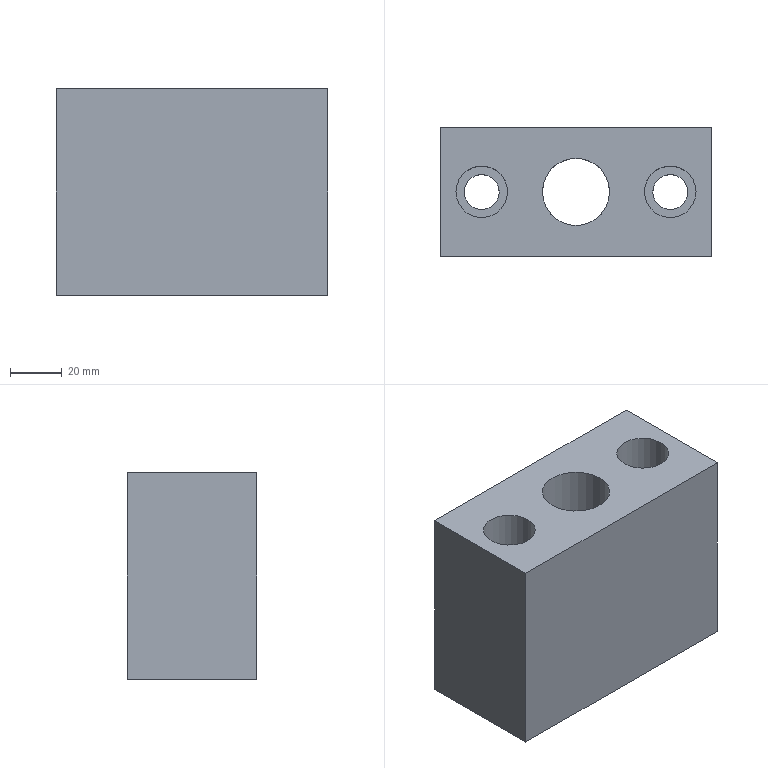Part | STEP file | lll_id1742_x_t | 1 solid | 15 faces | box 105 x 50 x 80 mm | volume 318087 mm3 | plane 9 | cylinder 6 | commonest cylinder face diameters 13.509 x2 20.007 x2 26 x1 38 x1
STEP:
#1=CARTESIAN_POINT('',(882.69,385.,87.5));
#2=VERTEX_POINT('',#1);
#3=CARTESIAN_POINT('',(875.935,385.,87.5));
#4=DIRECTION('',(0.,0.,1.));
#5=DIRECTION('',(1.,0.,0.));
#6=AXIS2_PLACEMENT_3D('',#3,#4,#5);
#7=CIRCLE('',#6,6.755);
#8=EDGE_CURVE('',#2,#2,#7,.T.);
#9=ORIENTED_EDGE('',*,*,#8,.F.);
#10=EDGE_LOOP('',(#9));
#11=FACE_BOUND('',#10,.T.);
#12=CARTESIAN_POINT('',(885.939,385.,87.5));
#13=VERTEX_POINT('',#12);
#14=CARTESIAN_POINT('',(875.935,385.,87.5));
#15=DIRECTION('',(0.,0.,1.));
#16=DIRECTION('',(1.,0.,0.));
#17=AXIS2_PLACEMENT_3D('',#14,#15,#16);
#18=CIRCLE('',#17,10.004);
#19=EDGE_CURVE('',#13,#13,#18,.T.);
#20=ORIENTED_EDGE('',*,*,#19,.T.);
#21=EDGE_LOOP('',(#20));
#22=FACE_BOUND('',#21,.T.);
#23=CARTESIAN_POINT('',(865.935,385.,87.5));
#24=DIRECTION('',(0.,0.,-1.));
#25=DIRECTION('',(1.,0.,0.));
#26=AXIS2_PLACEMENT_3D('',#23,#24,#25);
#27=PLANE('',#26);
#28=ADVANCED_FACE('',(#11,#22),#27,.F.);
#29=CARTESIAN_POINT('',(809.69,385.,87.5));
#30=VERTEX_POINT('',#29);
#31=CARTESIAN_POINT('',(802.935,385.,87.5));
#32=DIRECTION('',(0.,0.,1.));
#33=DIRECTION('',(1.,0.,0.));
#34=AXIS2_PLACEMENT_3D('',#31,#32,#33);
#35=CIRCLE('',#34,6.755);
#36=EDGE_CURVE('',#30,#30,#35,.T.);
#37=ORIENTED_EDGE('',*,*,#36,.F.);
#38=EDGE_LOOP('',(#37));
#39=FACE_BOUND('',#38,.T.);
#40=CARTESIAN_POINT('',(812.939,385.,87.5));
#41=VERTEX_POINT('',#40);
#42=CARTESIAN_POINT('',(802.935,385.,87.5));
#43=DIRECTION('',(0.,0.,1.));
#44=DIRECTION('',(1.,0.,0.));
#45=AXIS2_PLACEMENT_3D('',#42,#43,#44);
#46=CIRCLE('',#45,10.004);
#47=EDGE_CURVE('',#41,#41,#46,.T.);
#48=ORIENTED_EDGE('',*,*,#47,.T.);
#49=EDGE_LOOP('',(#48));
#50=FACE_BOUND('',#49,.T.);
#51=CARTESIAN_POINT('',(802.935,385.,87.5));
#52=DIRECTION('',(0.,0.,-1.));
#53=DIRECTION('',(1.,0.,0.));
#54=AXIS2_PLACEMENT_3D('',#51,#52,#53);
#55=PLANE('',#54);
#56=ADVANCED_FACE('',(#39,#50),#55,.F.);
#57=CARTESIAN_POINT('',(852.435,385.,132.5));
#58=VERTEX_POINT('',#57);
#59=CARTESIAN_POINT('',(839.435,385.,132.5));
#60=DIRECTION('',(0.,0.,1.));
#61=DIRECTION('',(1.,0.,0.));
#62=AXIS2_PLACEMENT_3D('',#59,#60,#61);
#63=CIRCLE('',#62,13.);
#64=EDGE_CURVE('',#58,#58,#63,.T.);
#65=ORIENTED_EDGE('',*,*,#64,.F.);
#66=EDGE_LOOP('',(#65));
#67=FACE_BOUND('',#66,.T.);
#68=CARTESIAN_POINT('',(885.939,385.,132.5));
#69=VERTEX_POINT('',#68);
#70=CARTESIAN_POINT('',(875.935,385.,132.5));
#71=DIRECTION('',(0.,0.,1.));
#72=DIRECTION('',(1.,0.,0.));
#73=AXIS2_PLACEMENT_3D('',#70,#71,#72);
#74=CIRCLE('',#73,10.004);
#75=EDGE_CURVE('',#69,#69,#74,.T.);
#76=ORIENTED_EDGE('',*,*,#75,.F.);
#77=EDGE_LOOP('',(#76));
#78=FACE_BOUND('',#77,.T.);
#79=CARTESIAN_POINT('',(891.935,360.,132.5));
#80=VERTEX_POINT('',#79);
#81=CARTESIAN_POINT('',(891.935,410.,132.5));
#82=VERTEX_POINT('',#81);
#83=CARTESIAN_POINT('',(891.935,385.,132.5));
#84=DIRECTION('',(0.,1.,0.));
#85=VECTOR('',#84,1.);
#86=LINE('',#83,#85);
#87=EDGE_CURVE('',#80,#82,#86,.T.);
#88=ORIENTED_EDGE('',*,*,#87,.T.);
#89=CARTESIAN_POINT('',(786.935,410.,132.5));
#90=VERTEX_POINT('',#89);
#91=CARTESIAN_POINT('',(839.435,410.,132.5));
#92=DIRECTION('',(-1.,0.,0.));
#93=VECTOR('',#92,1.);
#94=LINE('',#91,#93);
#95=EDGE_CURVE('',#82,#90,#94,.T.);
#96=ORIENTED_EDGE('',*,*,#95,.T.);
#97=CARTESIAN_POINT('',(786.935,360.,132.5));
#98=VERTEX_POINT('',#97);
#99=CARTESIAN_POINT('',(786.935,385.,132.5));
#100=DIRECTION('',(0.,-1.,0.));
#101=VECTOR('',#100,1.);
#102=LINE('',#99,#101);
#103=EDGE_CURVE('',#90,#98,#102,.T.);
#104=ORIENTED_EDGE('',*,*,#103,.T.);
#105=CARTESIAN_POINT('',(839.435,360.,132.5));
#106=DIRECTION('',(1.,0.,0.));
#107=VECTOR('',#106,1.);
#108=LINE('',#105,#107);
#109=EDGE_CURVE('',#98,#80,#108,.T.);
#110=ORIENTED_EDGE('',*,*,#109,.T.);
#111=EDGE_LOOP('',(#88,#96,#104,#110));
#112=FACE_BOUND('',#111,.T.);
#113=CARTESIAN_POINT('',(812.939,385.,132.5));
#114=VERTEX_POINT('',#113);
#115=CARTESIAN_POINT('',(802.935,385.,132.5));
#116=DIRECTION('',(0.,0.,1.));
#117=DIRECTION('',(1.,0.,0.));
#118=AXIS2_PLACEMENT_3D('',#115,#116,#117);
#119=CIRCLE('',#118,10.004);
#120=EDGE_CURVE('',#114,#114,#119,.T.);
#121=ORIENTED_EDGE('',*,*,#120,.F.);
#122=EDGE_LOOP('',(#121));
#123=FACE_BOUND('',#122,.T.);
#124=CARTESIAN_POINT('',(839.435,385.,132.5));
#125=DIRECTION('',(0.,0.,1.));
#126=DIRECTION('',(-1.,0.,0.));
#127=AXIS2_PLACEMENT_3D('',#124,#125,#126);
#128=PLANE('',#127);
#129=ADVANCED_FACE('',(#67,#78,#112,#123),#128,.T.);
#130=CARTESIAN_POINT('',(820.435,385.,52.5));
#131=VERTEX_POINT('',#130);
#132=CARTESIAN_POINT('',(839.435,385.,52.5));
#133=DIRECTION('',(0.,0.,-1.));
#134=DIRECTION('',(-1.,0.,0.));
#135=AXIS2_PLACEMENT_3D('',#132,#133,#134);
#136=CIRCLE('',#135,19.);
#137=EDGE_CURVE('',#131,#131,#136,.T.);
#138=ORIENTED_EDGE('',*,*,#137,.F.);
#139=EDGE_LOOP('',(#138));
#140=FACE_BOUND('',#139,.T.);
#141=CARTESIAN_POINT('',(882.69,385.,52.5));
#142=VERTEX_POINT('',#141);
#143=CARTESIAN_POINT('',(875.935,385.,52.5));
#144=DIRECTION('',(0.,0.,1.));
#145=DIRECTION('',(1.,0.,0.));
#146=AXIS2_PLACEMENT_3D('',#143,#144,#145);
#147=CIRCLE('',#146,6.755);
#148=EDGE_CURVE('',#142,#142,#147,.T.);
#149=ORIENTED_EDGE('',*,*,#148,.T.);
#150=EDGE_LOOP('',(#149));
#151=FACE_BOUND('',#150,.T.);
#152=CARTESIAN_POINT('',(809.69,385.,52.5));
#153=VERTEX_POINT('',#152);
#154=CARTESIAN_POINT('',(802.935,385.,52.5));
#155=DIRECTION('',(0.,0.,1.));
#156=DIRECTION('',(1.,0.,0.));
#157=AXIS2_PLACEMENT_3D('',#154,#155,#156);
#158=CIRCLE('',#157,6.755);
#159=EDGE_CURVE('',#153,#153,#158,.T.);
#160=ORIENTED_EDGE('',*,*,#159,.T.);
#161=EDGE_LOOP('',(#160));
#162=FACE_BOUND('',#161,.T.);
#163=CARTESIAN_POINT('',(891.935,360.,52.5));
#164=VERTEX_POINT('',#163);
#165=CARTESIAN_POINT('',(786.935,360.,52.5));
#166=VERTEX_POINT('',#165);
#167=CARTESIAN_POINT('',(839.435,360.,52.5));
#168=DIRECTION('',(-1.,0.,0.));
#169=VECTOR('',#168,1.);
#170=LINE('',#167,#169);
#171=EDGE_CURVE('',#164,#166,#170,.T.);
#172=ORIENTED_EDGE('',*,*,#171,.T.);
#173=CARTESIAN_POINT('',(786.935,410.,52.5));
#174=VERTEX_POINT('',#173);
#175=CARTESIAN_POINT('',(786.935,385.,52.5));
#176=DIRECTION('',(0.,1.,0.));
#177=VECTOR('',#176,1.);
#178=LINE('',#175,#177);
#179=EDGE_CURVE('',#166,#174,#178,.T.);
#180=ORIENTED_EDGE('',*,*,#179,.T.);
#181=CARTESIAN_POINT('',(891.935,410.,52.5));
#182=VERTEX_POINT('',#181);
#183=CARTESIAN_POINT('',(839.435,410.,52.5));
#184=DIRECTION('',(1.,0.,0.));
#185=VECTOR('',#184,1.);
#186=LINE('',#183,#185);
#187=EDGE_CURVE('',#174,#182,#186,.T.);
#188=ORIENTED_EDGE('',*,*,#187,.T.);
#189=CARTESIAN_POINT('',(891.935,385.,52.5));
#190=DIRECTION('',(0.,-1.,0.));
#191=VECTOR('',#190,1.);
#192=LINE('',#189,#191);
#193=EDGE_CURVE('',#182,#164,#192,.T.);
#194=ORIENTED_EDGE('',*,*,#193,.T.);
#195=EDGE_LOOP('',(#172,#180,#188,#194));
#196=FACE_BOUND('',#195,.T.);
#197=CARTESIAN_POINT('',(839.435,385.,52.5));
#198=DIRECTION('',(0.,0.,-1.));
#199=DIRECTION('',(1.,0.,0.));
#200=AXIS2_PLACEMENT_3D('',#197,#198,#199);
#201=PLANE('',#200);
#202=ADVANCED_FACE('',(#140,#151,#162,#196),#201,.T.);
#203=CARTESIAN_POINT('',(891.935,360.,132.5));
#204=DIRECTION('',(0.,0.,-1.));
#205=VECTOR('',#204,1.);
#206=LINE('',#203,#205);
#207=EDGE_CURVE('',#80,#164,#206,.T.);
#208=ORIENTED_EDGE('',*,*,#207,.F.);
#209=ORIENTED_EDGE('',*,*,#109,.F.);
#210=CARTESIAN_POINT('',(786.935,360.,132.5));
#211=DIRECTION('',(0.,0.,-1.));
#212=VECTOR('',#211,1.);
#213=LINE('',#210,#212);
#214=EDGE_CURVE('',#98,#166,#213,.T.);
#215=ORIENTED_EDGE('',*,*,#214,.T.);
#216=ORIENTED_EDGE('',*,*,#171,.F.);
#217=EDGE_LOOP('',(#208,#209,#215,#216));
#218=FACE_OUTER_BOUND('',#217,.T.);
#219=CARTESIAN_POINT('',(839.435,360.,132.5));
#220=DIRECTION('',(0.,-1.,0.));
#221=DIRECTION('',(0.,0.,1.));
#222=AXIS2_PLACEMENT_3D('',#219,#220,#221);
#223=PLANE('',#222);
#224=ADVANCED_FACE('',(#218),#223,.T.);
#225=ORIENTED_EDGE('',*,*,#214,.F.);
#226=ORIENTED_EDGE('',*,*,#103,.F.);
#227=CARTESIAN_POINT('',(786.935,410.,132.5));
#228=DIRECTION('',(0.,0.,-1.));
#229=VECTOR('',#228,1.);
#230=LINE('',#227,#229);
#231=EDGE_CURVE('',#90,#174,#230,.T.);
#232=ORIENTED_EDGE('',*,*,#231,.T.);
#233=ORIENTED_EDGE('',*,*,#179,.F.);
#234=EDGE_LOOP('',(#225,#226,#232,#233));
#235=FACE_OUTER_BOUND('',#234,.T.);
#236=CARTESIAN_POINT('',(786.935,385.,132.5));
#237=DIRECTION('',(-1.,0.,0.));
#238=DIRECTION('',(0.,0.,-1.));
#239=AXIS2_PLACEMENT_3D('',#236,#237,#238);
#240=PLANE('',#239);
#241=ADVANCED_FACE('',(#235),#240,.T.);
#242=ORIENTED_EDGE('',*,*,#231,.F.);
#243=ORIENTED_EDGE('',*,*,#95,.F.);
#244=CARTESIAN_POINT('',(891.935,410.,132.5));
#245=DIRECTION('',(0.,0.,-1.));
#246=VECTOR('',#245,1.);
#247=LINE('',#244,#246);
#248=EDGE_CURVE('',#82,#182,#247,.T.);
#249=ORIENTED_EDGE('',*,*,#248,.T.);
#250=ORIENTED_EDGE('',*,*,#187,.F.);
#251=EDGE_LOOP('',(#242,#243,#249,#250));
#252=FACE_OUTER_BOUND('',#251,.T.);
#253=CARTESIAN_POINT('',(839.435,410.,132.5));
#254=DIRECTION('',(0.,1.,0.));
#255=DIRECTION('',(0.,0.,-1.));
#256=AXIS2_PLACEMENT_3D('',#253,#254,#255);
#257=PLANE('',#256);
#258=ADVANCED_FACE('',(#252),#257,.T.);
#259=ORIENTED_EDGE('',*,*,#87,.F.);
#260=ORIENTED_EDGE('',*,*,#207,.T.);
#261=ORIENTED_EDGE('',*,*,#193,.F.);
#262=ORIENTED_EDGE('',*,*,#248,.F.);
#263=EDGE_LOOP('',(#259,#260,#261,#262));
#264=FACE_OUTER_BOUND('',#263,.T.);
#265=CARTESIAN_POINT('',(891.935,385.,132.5));
#266=DIRECTION('',(1.,0.,0.));
#267=DIRECTION('',(0.,0.,1.));
#268=AXIS2_PLACEMENT_3D('',#265,#266,#267);
#269=PLANE('',#268);
#270=ADVANCED_FACE('',(#264),#269,.T.);
#271=ORIENTED_EDGE('',*,*,#159,.F.);
#272=EDGE_LOOP('',(#271));
#273=FACE_BOUND('',#272,.T.);
#274=ORIENTED_EDGE('',*,*,#36,.T.);
#275=EDGE_LOOP('',(#274));
#276=FACE_BOUND('',#275,.T.);
#277=CARTESIAN_POINT('',(802.935,385.,137.5));
#278=DIRECTION('',(0.,0.,-1.));
#279=DIRECTION('',(1.,0.,0.));
#280=AXIS2_PLACEMENT_3D('',#277,#278,#279);
#281=CYLINDRICAL_SURFACE('',#280,6.755);
#282=ADVANCED_FACE('',(#273,#276),#281,.F.);
#283=ORIENTED_EDGE('',*,*,#47,.F.);
#284=EDGE_LOOP('',(#283));
#285=FACE_BOUND('',#284,.T.);
#286=ORIENTED_EDGE('',*,*,#120,.T.);
#287=EDGE_LOOP('',(#286));
#288=FACE_BOUND('',#287,.T.);
#289=CARTESIAN_POINT('',(802.935,385.,132.5));
#290=DIRECTION('',(0.,0.,-1.));
#291=DIRECTION('',(1.,0.,0.));
#292=AXIS2_PLACEMENT_3D('',#289,#290,#291);
#293=CYLINDRICAL_SURFACE('',#292,10.004);
#294=ADVANCED_FACE('',(#285,#288),#293,.F.);
#295=ORIENTED_EDGE('',*,*,#148,.F.);
#296=EDGE_LOOP('',(#295));
#297=FACE_BOUND('',#296,.T.);
#298=ORIENTED_EDGE('',*,*,#8,.T.);
#299=EDGE_LOOP('',(#298));
#300=FACE_BOUND('',#299,.T.);
#301=CARTESIAN_POINT('',(875.935,385.,137.5));
#302=DIRECTION('',(0.,0.,-1.));
#303=DIRECTION('',(1.,0.,0.));
#304=AXIS2_PLACEMENT_3D('',#301,#302,#303);
#305=CYLINDRICAL_SURFACE('',#304,6.755);
#306=ADVANCED_FACE('',(#297,#300),#305,.F.);
#307=ORIENTED_EDGE('',*,*,#19,.F.);
#308=EDGE_LOOP('',(#307));
#309=FACE_BOUND('',#308,.T.);
#310=ORIENTED_EDGE('',*,*,#75,.T.);
#311=EDGE_LOOP('',(#310));
#312=FACE_BOUND('',#311,.T.);
#313=CARTESIAN_POINT('',(875.935,385.,132.5));
#314=DIRECTION('',(0.,0.,-1.));
#315=DIRECTION('',(1.,0.,0.));
#316=AXIS2_PLACEMENT_3D('',#313,#314,#315);
#317=CYLINDRICAL_SURFACE('',#316,10.004);
#318=ADVANCED_FACE('',(#309,#312),#317,.F.);
#319=CARTESIAN_POINT('',(826.435,385.,87.5));
#320=VERTEX_POINT('',#319);
#321=CARTESIAN_POINT('',(839.435,385.,87.5));
#322=DIRECTION('',(0.,0.,-1.));
#323=DIRECTION('',(-1.,0.,0.));
#324=AXIS2_PLACEMENT_3D('',#321,#322,#323);
#325=CIRCLE('',#324,13.);
#326=EDGE_CURVE('',#320,#320,#325,.T.);
#327=ORIENTED_EDGE('',*,*,#326,.F.);
#328=EDGE_LOOP('',(#327));
#329=FACE_BOUND('',#328,.T.);
#330=CARTESIAN_POINT('',(820.435,385.,87.5));
#331=VERTEX_POINT('',#330);
#332=CARTESIAN_POINT('',(839.435,385.,87.5));
#333=DIRECTION('',(0.,0.,1.));
#334=DIRECTION('',(-1.,0.,0.));
#335=AXIS2_PLACEMENT_3D('',#332,#333,#334);
#336=CIRCLE('',#335,19.);
#337=EDGE_CURVE('',#331,#331,#336,.T.);
#338=ORIENTED_EDGE('',*,*,#337,.F.);
#339=EDGE_LOOP('',(#338));
#340=FACE_BOUND('',#339,.T.);
#341=CARTESIAN_POINT('',(839.435,385.,87.5));
#342=DIRECTION('',(0.,0.,-1.));
#343=DIRECTION('',(-1.,0.,0.));
#344=AXIS2_PLACEMENT_3D('',#341,#342,#343);
#345=PLANE('',#344);
#346=ADVANCED_FACE('',(#329,#340),#345,.T.);
#347=ORIENTED_EDGE('',*,*,#137,.T.);
#348=EDGE_LOOP('',(#347));
#349=FACE_BOUND('',#348,.T.);
#350=ORIENTED_EDGE('',*,*,#337,.T.);
#351=EDGE_LOOP('',(#350));
#352=FACE_BOUND('',#351,.T.);
#353=CARTESIAN_POINT('',(839.435,385.,87.5));
#354=DIRECTION('',(0.,0.,-1.));
#355=DIRECTION('',(-1.,0.,0.));
#356=AXIS2_PLACEMENT_3D('',#353,#354,#355);
#357=CYLINDRICAL_SURFACE('',#356,19.);
#358=ADVANCED_FACE('',(#349,#352),#357,.F.);
#359=ORIENTED_EDGE('',*,*,#64,.T.);
#360=EDGE_LOOP('',(#359));
#361=FACE_BOUND('',#360,.T.);
#362=ORIENTED_EDGE('',*,*,#326,.T.);
#363=EDGE_LOOP('',(#362));
#364=FACE_BOUND('',#363,.T.);
#365=CARTESIAN_POINT('',(839.435,385.,37.5));
#366=DIRECTION('',(0.,0.,1.));
#367=DIRECTION('',(1.,0.,0.));
#368=AXIS2_PLACEMENT_3D('',#365,#366,#367);
#369=CYLINDRICAL_SURFACE('',#368,13.);
#370=ADVANCED_FACE('',(#361,#364),#369,.F.);
#371=CLOSED_SHELL('',(#28,#56,#129,#202,#224,#241,#258,#270,#282,#294,#306,#318,#346,#358,#370));
#372=MANIFOLD_SOLID_BREP('',#371);
#373=(LENGTH_UNIT()NAMED_UNIT(*)SI_UNIT(.MILLI.,.METRE.));
#374=UNCERTAINTY_MEASURE_WITH_UNIT(LENGTH_MEASURE(0.00002),#373,'','');
#375=(NAMED_UNIT(*)PLANE_ANGLE_UNIT()SI_UNIT($,.RADIAN.));
#376=PLANE_ANGLE_MEASURE_WITH_UNIT(PLANE_ANGLE_MEASURE(0.01745),#375);
#377=DIMENSIONAL_EXPONENTS(0.,0.,0.,0.,0.,0.,0.);
#378=(CONVERSION_BASED_UNIT('DEGREE',#376)NAMED_UNIT(#377)PLANE_ANGLE_UNIT());
#379=(NAMED_UNIT(*)SI_UNIT($,.STERADIAN.)SOLID_ANGLE_UNIT());
#380=(GEOMETRIC_REPRESENTATION_CONTEXT(3)GLOBAL_UNCERTAINTY_ASSIGNED_CONTEXT((#374))GLOBAL_UNIT_ASSIGNED_CONTEXT((#373,#378,#379))REPRESENTATION_CONTEXT('',''));
#381=ADVANCED_BREP_SHAPE_REPRESENTATION('',(#372),#380);